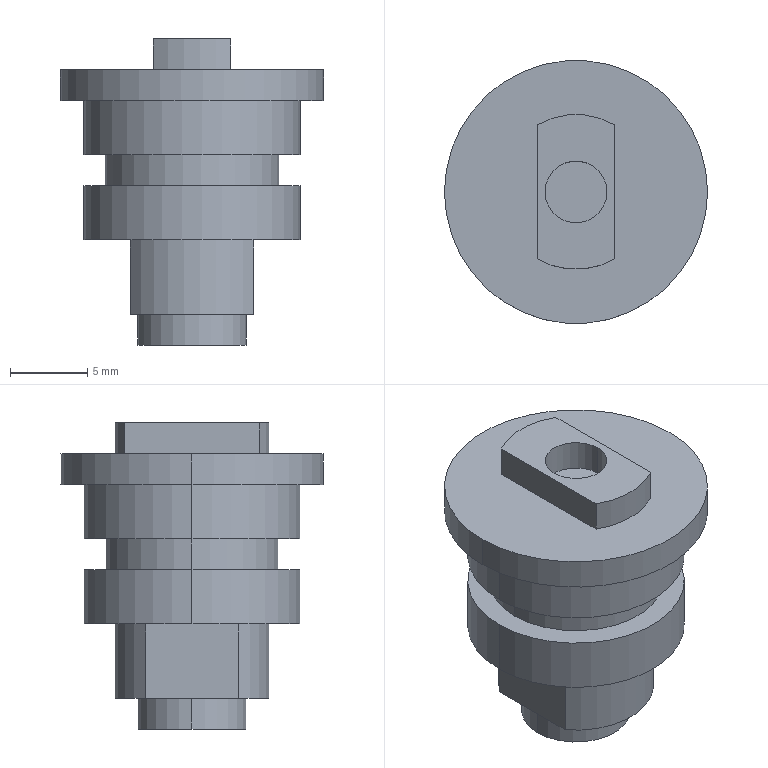Part | SolidWorks | features ICE 3, HoleWzd 1, Revolution 1 | 1 solid | 35 faces | box 17 x 17 x 19.8 mm | volume 2110 mm3 | cylinder 18 | plane 13 | cone 4 | commonest cylinder face diameters 10 x4 14 x4 4 x2 4.2 x2 7 x2 11.2 x2
STEP:
#1=CARTESIAN_POINT('',(-2.,0.,-2.));
#2=VERTEX_POINT('',#1);
#3=CARTESIAN_POINT('',(2.,0.,-2.));
#4=VERTEX_POINT('',#3);
#5=CARTESIAN_POINT('',(0.,0.,-2.));
#6=DIRECTION('',(0.,0.,1.));
#7=DIRECTION('',(1.,0.,0.));
#8=AXIS2_PLACEMENT_3D('',#5,#6,#7);
#9=CIRCLE('',#8,2.);
#10=EDGE_CURVE('',#2,#4,#9,.T.);
#11=ORIENTED_EDGE('',*,*,#10,.F.);
#12=CARTESIAN_POINT('',(-2.,0.,0.));
#13=VERTEX_POINT('',#12);
#14=CARTESIAN_POINT('',(-2.,0.,-2.));
#15=DIRECTION('',(0.,0.,1.));
#16=VECTOR('',#15,1000.);
#17=LINE('',#14,#16);
#18=EDGE_CURVE('',#2,#13,#17,.T.);
#19=ORIENTED_EDGE('',*,*,#18,.T.);
#20=CARTESIAN_POINT('',(2.,0.,0.));
#21=VERTEX_POINT('',#20);
#22=CARTESIAN_POINT('',(0.,0.,0.));
#23=DIRECTION('',(0.,0.,1.));
#24=DIRECTION('',(1.,0.,0.));
#25=AXIS2_PLACEMENT_3D('',#22,#23,#24);
#26=CIRCLE('',#25,2.);
#27=EDGE_CURVE('',#13,#21,#26,.T.);
#28=ORIENTED_EDGE('',*,*,#27,.T.);
#29=CARTESIAN_POINT('',(2.,0.,-2.));
#30=DIRECTION('',(0.,0.,1.));
#31=VECTOR('',#30,1000.);
#32=LINE('',#29,#31);
#33=EDGE_CURVE('',#4,#21,#32,.T.);
#34=ORIENTED_EDGE('',*,*,#33,.F.);
#35=EDGE_LOOP('',(#11,#19,#28,#34));
#36=FACE_OUTER_BOUND('',#35,.T.);
#37=CARTESIAN_POINT('',(0.,0.,-2.));
#38=DIRECTION('',(0.,0.,1.));
#39=DIRECTION('',(1.,0.,0.));
#40=AXIS2_PLACEMENT_3D('',#37,#38,#39);
#41=CYLINDRICAL_SURFACE('',#40,2.);
#42=ADVANCED_FACE('',(#36),#41,.F.);
#43=CARTESIAN_POINT('',(2.1,0.,-19.375));
#44=VERTEX_POINT('',#43);
#45=CARTESIAN_POINT('',(-2.1,0.,-19.375));
#46=VERTEX_POINT('',#45);
#47=CARTESIAN_POINT('',(0.,0.,-19.375));
#48=DIRECTION('',(0.,0.,-1.));
#49=DIRECTION('',(-1.,0.,0.));
#50=AXIS2_PLACEMENT_3D('',#47,#48,#49);
#51=CIRCLE('',#50,2.1);
#52=EDGE_CURVE('',#44,#46,#51,.T.);
#53=ORIENTED_EDGE('',*,*,#52,.F.);
#54=CARTESIAN_POINT('',(2.525,0.,-19.8));
#55=VERTEX_POINT('',#54);
#56=CARTESIAN_POINT('',(2.525,0.,-19.8));
#57=DIRECTION('',(0.7071,0.,-0.7071));
#58=VECTOR('',#57,1000.);
#59=LINE('',#56,#58);
#60=EDGE_CURVE('',#44,#55,#59,.T.);
#61=ORIENTED_EDGE('',*,*,#60,.T.);
#62=CARTESIAN_POINT('',(-2.525,0.,-19.8));
#63=VERTEX_POINT('',#62);
#64=CARTESIAN_POINT('',(0.,0.,-19.8));
#65=DIRECTION('',(0.,0.,-1.));
#66=DIRECTION('',(-1.,0.,0.));
#67=AXIS2_PLACEMENT_3D('',#64,#65,#66);
#68=CIRCLE('',#67,2.525);
#69=EDGE_CURVE('',#55,#63,#68,.T.);
#70=ORIENTED_EDGE('',*,*,#69,.T.);
#71=CARTESIAN_POINT('',(-2.525,0.,-19.8));
#72=DIRECTION('',(-0.7071,0.,-0.7071));
#73=VECTOR('',#72,1000.);
#74=LINE('',#71,#73);
#75=EDGE_CURVE('',#46,#63,#74,.T.);
#76=ORIENTED_EDGE('',*,*,#75,.F.);
#77=EDGE_LOOP('',(#53,#61,#70,#76));
#78=FACE_OUTER_BOUND('',#77,.T.);
#79=CARTESIAN_POINT('',(0.,0.,-19.8));
#80=DIRECTION('',(0.,0.,-1.));
#81=DIRECTION('',(-1.,0.,0.));
#82=AXIS2_PLACEMENT_3D('',#79,#80,#81);
#83=CONICAL_SURFACE('',#82,2.525,0.7854);
#84=ADVANCED_FACE('',(#78),#83,.F.);
#85=CARTESIAN_POINT('',(2.1,0.,-12.8));
#86=VERTEX_POINT('',#85);
#87=CARTESIAN_POINT('',(-2.1,0.,-12.8));
#88=VERTEX_POINT('',#87);
#89=CARTESIAN_POINT('',(0.,0.,-12.8));
#90=DIRECTION('',(0.,0.,-1.));
#91=DIRECTION('',(-1.,0.,0.));
#92=AXIS2_PLACEMENT_3D('',#89,#90,#91);
#93=CIRCLE('',#92,2.1);
#94=EDGE_CURVE('',#86,#88,#93,.T.);
#95=ORIENTED_EDGE('',*,*,#94,.F.);
#96=CARTESIAN_POINT('',(2.1,0.,-19.8));
#97=DIRECTION('',(0.,0.,-1.));
#98=VECTOR('',#97,1000.);
#99=LINE('',#96,#98);
#100=EDGE_CURVE('',#86,#44,#99,.T.);
#101=ORIENTED_EDGE('',*,*,#100,.T.);
#102=ORIENTED_EDGE('',*,*,#52,.T.);
#103=CARTESIAN_POINT('',(-2.1,0.,-19.8));
#104=DIRECTION('',(0.,0.,-1.));
#105=VECTOR('',#104,1000.);
#106=LINE('',#103,#105);
#107=EDGE_CURVE('',#88,#46,#106,.T.);
#108=ORIENTED_EDGE('',*,*,#107,.F.);
#109=EDGE_LOOP('',(#95,#101,#102,#108));
#110=FACE_OUTER_BOUND('',#109,.T.);
#111=CARTESIAN_POINT('',(0.,0.,-19.8));
#112=DIRECTION('',(0.,0.,-1.));
#113=DIRECTION('',(-1.,0.,0.));
#114=AXIS2_PLACEMENT_3D('',#111,#112,#113);
#115=CYLINDRICAL_SURFACE('',#114,2.1);
#116=ADVANCED_FACE('',(#110),#115,.F.);
#117=CARTESIAN_POINT('',(0.,0.,-11.538));
#118=VERTEX_POINT('',#117);
#119=CARTESIAN_POINT('',(-2.1,0.,-12.8));
#120=DIRECTION('',(-0.8572,0.,-0.515));
#121=VECTOR('',#120,1000.);
#122=LINE('',#119,#121);
#123=EDGE_CURVE('',#118,#88,#122,.T.);
#124=ORIENTED_EDGE('',*,*,#123,.F.);
#125=CARTESIAN_POINT('',(2.1,0.,-12.8));
#126=DIRECTION('',(0.8572,0.,-0.515));
#127=VECTOR('',#126,1000.);
#128=LINE('',#125,#127);
#129=EDGE_CURVE('',#118,#86,#128,.T.);
#130=ORIENTED_EDGE('',*,*,#129,.T.);
#131=ORIENTED_EDGE('',*,*,#94,.T.);
#132=EDGE_LOOP('',(#124,#130,#131));
#133=FACE_OUTER_BOUND('',#132,.T.);
#134=CARTESIAN_POINT('',(0.,0.,-12.8));
#135=DIRECTION('',(0.,0.,-1.));
#136=DIRECTION('',(-1.,0.,0.));
#137=AXIS2_PLACEMENT_3D('',#134,#135,#136);
#138=CONICAL_SURFACE('',#137,2.1,1.03);
#139=ADVANCED_FACE('',(#133),#138,.F.);
#140=CARTESIAN_POINT('',(-3.5,0.,-17.8));
#141=VERTEX_POINT('',#140);
#142=CARTESIAN_POINT('',(3.5,0.,-17.8));
#143=VERTEX_POINT('',#142);
#144=CARTESIAN_POINT('',(0.,0.,-17.8));
#145=DIRECTION('',(0.,0.,-1.));
#146=DIRECTION('',(-1.,0.,0.));
#147=AXIS2_PLACEMENT_3D('',#144,#145,#146);
#148=CIRCLE('',#147,3.5);
#149=EDGE_CURVE('',#141,#143,#148,.T.);
#150=ORIENTED_EDGE('',*,*,#149,.T.);
#151=CARTESIAN_POINT('',(3.5,0.,-19.8));
#152=VERTEX_POINT('',#151);
#153=CARTESIAN_POINT('',(3.5,0.,-19.8));
#154=DIRECTION('',(0.,0.,-1.));
#155=VECTOR('',#154,1000.);
#156=LINE('',#153,#155);
#157=EDGE_CURVE('',#143,#152,#156,.T.);
#158=ORIENTED_EDGE('',*,*,#157,.T.);
#159=CARTESIAN_POINT('',(-3.5,0.,-19.8));
#160=VERTEX_POINT('',#159);
#161=CARTESIAN_POINT('',(0.,0.,-19.8));
#162=DIRECTION('',(0.,0.,-1.));
#163=DIRECTION('',(-1.,0.,0.));
#164=AXIS2_PLACEMENT_3D('',#161,#162,#163);
#165=CIRCLE('',#164,3.5);
#166=EDGE_CURVE('',#160,#152,#165,.T.);
#167=ORIENTED_EDGE('',*,*,#166,.F.);
#168=CARTESIAN_POINT('',(-3.5,0.,-19.8));
#169=DIRECTION('',(0.,0.,-1.));
#170=VECTOR('',#169,1000.);
#171=LINE('',#168,#170);
#172=EDGE_CURVE('',#141,#160,#171,.T.);
#173=ORIENTED_EDGE('',*,*,#172,.F.);
#174=EDGE_LOOP('',(#150,#158,#167,#173));
#175=FACE_OUTER_BOUND('',#174,.T.);
#176=CARTESIAN_POINT('',(0.,0.,-19.8));
#177=DIRECTION('',(0.,0.,-1.));
#178=DIRECTION('',(-1.,0.,0.));
#179=AXIS2_PLACEMENT_3D('',#176,#177,#178);
#180=CYLINDRICAL_SURFACE('',#179,3.5);
#181=ADVANCED_FACE('',(#175),#180,.T.);
#182=CARTESIAN_POINT('',(-7.,0.,-9.5));
#183=VERTEX_POINT('',#182);
#184=CARTESIAN_POINT('',(7.,0.,-9.5));
#185=VERTEX_POINT('',#184);
#186=CARTESIAN_POINT('',(0.,0.,-9.5));
#187=DIRECTION('',(0.,0.,-1.));
#188=DIRECTION('',(-1.,0.,0.));
#189=AXIS2_PLACEMENT_3D('',#186,#187,#188);
#190=CIRCLE('',#189,7.);
#191=EDGE_CURVE('',#183,#185,#190,.T.);
#192=ORIENTED_EDGE('',*,*,#191,.T.);
#193=CARTESIAN_POINT('',(7.,0.,-13.));
#194=VERTEX_POINT('',#193);
#195=CARTESIAN_POINT('',(7.,0.,-19.8));
#196=DIRECTION('',(0.,0.,-1.));
#197=VECTOR('',#196,1000.);
#198=LINE('',#195,#197);
#199=EDGE_CURVE('',#185,#194,#198,.T.);
#200=ORIENTED_EDGE('',*,*,#199,.T.);
#201=CARTESIAN_POINT('',(-7.,0.,-13.));
#202=VERTEX_POINT('',#201);
#203=CARTESIAN_POINT('',(0.,0.,-13.));
#204=DIRECTION('',(0.,0.,-1.));
#205=DIRECTION('',(-1.,0.,0.));
#206=AXIS2_PLACEMENT_3D('',#203,#204,#205);
#207=CIRCLE('',#206,7.);
#208=EDGE_CURVE('',#202,#194,#207,.T.);
#209=ORIENTED_EDGE('',*,*,#208,.F.);
#210=CARTESIAN_POINT('',(-7.,0.,-19.8));
#211=DIRECTION('',(0.,0.,-1.));
#212=VECTOR('',#211,1000.);
#213=LINE('',#210,#212);
#214=EDGE_CURVE('',#183,#202,#213,.T.);
#215=ORIENTED_EDGE('',*,*,#214,.F.);
#216=EDGE_LOOP('',(#192,#200,#209,#215));
#217=FACE_OUTER_BOUND('',#216,.T.);
#218=CARTESIAN_POINT('',(0.,0.,-19.8));
#219=DIRECTION('',(0.,0.,-1.));
#220=DIRECTION('',(-1.,0.,0.));
#221=AXIS2_PLACEMENT_3D('',#218,#219,#220);
#222=CYLINDRICAL_SURFACE('',#221,7.);
#223=ADVANCED_FACE('',(#217),#222,.T.);
#224=CARTESIAN_POINT('',(-5.6,0.,-7.5));
#225=VERTEX_POINT('',#224);
#226=CARTESIAN_POINT('',(5.6,0.,-7.5));
#227=VERTEX_POINT('',#226);
#228=CARTESIAN_POINT('',(0.,0.,-7.5));
#229=DIRECTION('',(0.,0.,-1.));
#230=DIRECTION('',(-1.,0.,0.));
#231=AXIS2_PLACEMENT_3D('',#228,#229,#230);
#232=CIRCLE('',#231,5.6);
#233=EDGE_CURVE('',#225,#227,#232,.T.);
#234=ORIENTED_EDGE('',*,*,#233,.T.);
#235=CARTESIAN_POINT('',(5.6,0.,-9.5));
#236=VERTEX_POINT('',#235);
#237=CARTESIAN_POINT('',(5.6,0.,-19.8));
#238=DIRECTION('',(0.,0.,-1.));
#239=VECTOR('',#238,1000.);
#240=LINE('',#237,#239);
#241=EDGE_CURVE('',#227,#236,#240,.T.);
#242=ORIENTED_EDGE('',*,*,#241,.T.);
#243=CARTESIAN_POINT('',(-5.6,0.,-9.5));
#244=VERTEX_POINT('',#243);
#245=CARTESIAN_POINT('',(0.,0.,-9.5));
#246=DIRECTION('',(0.,0.,-1.));
#247=DIRECTION('',(-1.,0.,0.));
#248=AXIS2_PLACEMENT_3D('',#245,#246,#247);
#249=CIRCLE('',#248,5.6);
#250=EDGE_CURVE('',#244,#236,#249,.T.);
#251=ORIENTED_EDGE('',*,*,#250,.F.);
#252=CARTESIAN_POINT('',(-5.6,0.,-19.8));
#253=DIRECTION('',(0.,0.,-1.));
#254=VECTOR('',#253,1000.);
#255=LINE('',#252,#254);
#256=EDGE_CURVE('',#225,#244,#255,.T.);
#257=ORIENTED_EDGE('',*,*,#256,.F.);
#258=EDGE_LOOP('',(#234,#242,#251,#257));
#259=FACE_OUTER_BOUND('',#258,.T.);
#260=CARTESIAN_POINT('',(0.,0.,-19.8));
#261=DIRECTION('',(0.,0.,-1.));
#262=DIRECTION('',(-1.,0.,0.));
#263=AXIS2_PLACEMENT_3D('',#260,#261,#262);
#264=CYLINDRICAL_SURFACE('',#263,5.6);
#265=ADVANCED_FACE('',(#259),#264,.T.);
#266=CARTESIAN_POINT('',(-7.,0.,-4.));
#267=VERTEX_POINT('',#266);
#268=CARTESIAN_POINT('',(7.,0.,-4.));
#269=VERTEX_POINT('',#268);
#270=CARTESIAN_POINT('',(0.,0.,-4.));
#271=DIRECTION('',(0.,0.,-1.));
#272=DIRECTION('',(-1.,0.,0.));
#273=AXIS2_PLACEMENT_3D('',#270,#271,#272);
#274=CIRCLE('',#273,7.);
#275=EDGE_CURVE('',#267,#269,#274,.T.);
#276=ORIENTED_EDGE('',*,*,#275,.T.);
#277=CARTESIAN_POINT('',(7.,0.,-7.5));
#278=VERTEX_POINT('',#277);
#279=CARTESIAN_POINT('',(7.,0.,-19.8));
#280=DIRECTION('',(0.,0.,-1.));
#281=VECTOR('',#280,1000.);
#282=LINE('',#279,#281);
#283=EDGE_CURVE('',#269,#278,#282,.T.);
#284=ORIENTED_EDGE('',*,*,#283,.T.);
#285=CARTESIAN_POINT('',(-7.,0.,-7.5));
#286=VERTEX_POINT('',#285);
#287=CARTESIAN_POINT('',(0.,0.,-7.5));
#288=DIRECTION('',(0.,0.,-1.));
#289=DIRECTION('',(-1.,0.,0.));
#290=AXIS2_PLACEMENT_3D('',#287,#288,#289);
#291=CIRCLE('',#290,7.);
#292=EDGE_CURVE('',#286,#278,#291,.T.);
#293=ORIENTED_EDGE('',*,*,#292,.F.);
#294=CARTESIAN_POINT('',(-7.,0.,-19.8));
#295=DIRECTION('',(0.,0.,-1.));
#296=VECTOR('',#295,1000.);
#297=LINE('',#294,#296);
#298=EDGE_CURVE('',#267,#286,#297,.T.);
#299=ORIENTED_EDGE('',*,*,#298,.F.);
#300=EDGE_LOOP('',(#276,#284,#293,#299));
#301=FACE_OUTER_BOUND('',#300,.T.);
#302=CARTESIAN_POINT('',(0.,0.,-19.8));
#303=DIRECTION('',(0.,0.,-1.));
#304=DIRECTION('',(-1.,0.,0.));
#305=AXIS2_PLACEMENT_3D('',#302,#303,#304);
#306=CYLINDRICAL_SURFACE('',#305,7.);
#307=ADVANCED_FACE('',(#301),#306,.T.);
#308=CARTESIAN_POINT('',(-8.5,0.,-2.));
#309=VERTEX_POINT('',#308);
#310=CARTESIAN_POINT('',(8.5,0.,-2.));
#311=VERTEX_POINT('',#310);
#312=CARTESIAN_POINT('',(0.,0.,-2.));
#313=DIRECTION('',(0.,0.,-1.));
#314=DIRECTION('',(-1.,0.,0.));
#315=AXIS2_PLACEMENT_3D('',#312,#313,#314);
#316=CIRCLE('',#315,8.5);
#317=EDGE_CURVE('',#309,#311,#316,.T.);
#318=ORIENTED_EDGE('',*,*,#317,.T.);
#319=CARTESIAN_POINT('',(8.5,0.,-4.));
#320=VERTEX_POINT('',#319);
#321=CARTESIAN_POINT('',(8.5,0.,-19.8));
#322=DIRECTION('',(0.,0.,-1.));
#323=VECTOR('',#322,1000.);
#324=LINE('',#321,#323);
#325=EDGE_CURVE('',#311,#320,#324,.T.);
#326=ORIENTED_EDGE('',*,*,#325,.T.);
#327=CARTESIAN_POINT('',(-8.5,0.,-4.));
#328=VERTEX_POINT('',#327);
#329=CARTESIAN_POINT('',(0.,0.,-4.));
#330=DIRECTION('',(0.,0.,-1.));
#331=DIRECTION('',(-1.,0.,0.));
#332=AXIS2_PLACEMENT_3D('',#329,#330,#331);
#333=CIRCLE('',#332,8.5);
#334=EDGE_CURVE('',#328,#320,#333,.T.);
#335=ORIENTED_EDGE('',*,*,#334,.F.);
#336=CARTESIAN_POINT('',(-8.5,0.,-19.8));
#337=DIRECTION('',(0.,0.,-1.));
#338=VECTOR('',#337,1000.);
#339=LINE('',#336,#338);
#340=EDGE_CURVE('',#309,#328,#339,.T.);
#341=ORIENTED_EDGE('',*,*,#340,.F.);
#342=EDGE_LOOP('',(#318,#326,#335,#341));
#343=FACE_OUTER_BOUND('',#342,.T.);
#344=CARTESIAN_POINT('',(0.,0.,-19.8));
#345=DIRECTION('',(0.,0.,-1.));
#346=DIRECTION('',(-1.,0.,0.));
#347=AXIS2_PLACEMENT_3D('',#344,#345,#346);
#348=CYLINDRICAL_SURFACE('',#347,8.5);
#349=ADVANCED_FACE('',(#343),#348,.T.);
#350=CARTESIAN_POINT('',(4.,-3.,-17.8));
#351=VERTEX_POINT('',#350);
#352=CARTESIAN_POINT('',(-4.,-3.,-17.8));
#353=VERTEX_POINT('',#352);
#354=CARTESIAN_POINT('',(0.,0.,-17.8));
#355=DIRECTION('',(0.,0.,-1.));
#356=DIRECTION('',(-1.,0.,0.));
#357=AXIS2_PLACEMENT_3D('',#354,#355,#356);
#358=CIRCLE('',#357,5.);
#359=EDGE_CURVE('',#351,#353,#358,.T.);
#360=ORIENTED_EDGE('',*,*,#359,.F.);
#361=CARTESIAN_POINT('',(4.,-3.,-13.));
#362=VERTEX_POINT('',#361);
#363=CARTESIAN_POINT('',(4.,-3.,-19.8));
#364=DIRECTION('',(0.,0.,1.));
#365=VECTOR('',#364,1000.);
#366=LINE('',#363,#365);
#367=EDGE_CURVE('',#351,#362,#366,.T.);
#368=ORIENTED_EDGE('',*,*,#367,.T.);
#369=CARTESIAN_POINT('',(-4.,-3.,-13.));
#370=VERTEX_POINT('',#369);
#371=CARTESIAN_POINT('',(0.,0.,-13.));
#372=DIRECTION('',(0.,0.,-1.));
#373=DIRECTION('',(-1.,0.,0.));
#374=AXIS2_PLACEMENT_3D('',#371,#372,#373);
#375=CIRCLE('',#374,5.);
#376=EDGE_CURVE('',#362,#370,#375,.T.);
#377=ORIENTED_EDGE('',*,*,#376,.T.);
#378=CARTESIAN_POINT('',(-4.,-3.,-19.8));
#379=DIRECTION('',(0.,0.,-1.));
#380=VECTOR('',#379,1000.);
#381=LINE('',#378,#380);
#382=EDGE_CURVE('',#370,#353,#381,.T.);
#383=ORIENTED_EDGE('',*,*,#382,.T.);
#384=EDGE_LOOP('',(#360,#368,#377,#383));
#385=FACE_OUTER_BOUND('',#384,.T.);
#386=CARTESIAN_POINT('',(0.,0.,-19.8));
#387=DIRECTION('',(0.,0.,-1.));
#388=DIRECTION('',(-1.,0.,0.));
#389=AXIS2_PLACEMENT_3D('',#386,#387,#388);
#390=CYLINDRICAL_SURFACE('',#389,5.);
#391=ADVANCED_FACE('',(#385),#390,.T.);
#392=CARTESIAN_POINT('',(-4.,3.,-13.));
#393=VERTEX_POINT('',#392);
#394=CARTESIAN_POINT('',(4.,3.,-13.));
#395=VERTEX_POINT('',#394);
#396=CARTESIAN_POINT('',(0.,0.,-13.));
#397=DIRECTION('',(0.,0.,-1.));
#398=DIRECTION('',(-1.,0.,0.));
#399=AXIS2_PLACEMENT_3D('',#396,#397,#398);
#400=CIRCLE('',#399,5.);
#401=EDGE_CURVE('',#393,#395,#400,.T.);
#402=ORIENTED_EDGE('',*,*,#401,.T.);
#403=CARTESIAN_POINT('',(4.,3.,-17.8));
#404=VERTEX_POINT('',#403);
#405=CARTESIAN_POINT('',(4.,3.,-19.8));
#406=DIRECTION('',(0.,0.,-1.));
#407=VECTOR('',#406,1000.);
#408=LINE('',#405,#407);
#409=EDGE_CURVE('',#395,#404,#408,.T.);
#410=ORIENTED_EDGE('',*,*,#409,.T.);
#411=CARTESIAN_POINT('',(-4.,3.,-17.8));
#412=VERTEX_POINT('',#411);
#413=CARTESIAN_POINT('',(0.,0.,-17.8));
#414=DIRECTION('',(0.,0.,-1.));
#415=DIRECTION('',(-1.,0.,0.));
#416=AXIS2_PLACEMENT_3D('',#413,#414,#415);
#417=CIRCLE('',#416,5.);
#418=EDGE_CURVE('',#412,#404,#417,.T.);
#419=ORIENTED_EDGE('',*,*,#418,.F.);
#420=CARTESIAN_POINT('',(-4.,3.,-19.8));
#421=DIRECTION('',(0.,0.,1.));
#422=VECTOR('',#421,1000.);
#423=LINE('',#420,#422);
#424=EDGE_CURVE('',#412,#393,#423,.T.);
#425=ORIENTED_EDGE('',*,*,#424,.T.);
#426=EDGE_LOOP('',(#402,#410,#419,#425));
#427=FACE_OUTER_BOUND('',#426,.T.);
#428=CARTESIAN_POINT('',(0.,0.,-19.8));
#429=DIRECTION('',(0.,0.,-1.));
#430=DIRECTION('',(-1.,0.,0.));
#431=AXIS2_PLACEMENT_3D('',#428,#429,#430);
#432=CYLINDRICAL_SURFACE('',#431,5.);
#433=ADVANCED_FACE('',(#427),#432,.T.);
#434=ORIENTED_EDGE('',*,*,#149,.F.);
#435=CARTESIAN_POINT('',(0.,0.,-17.8));
#436=DIRECTION('',(0.,0.,-1.));
#437=DIRECTION('',(-1.,0.,0.));
#438=AXIS2_PLACEMENT_3D('',#435,#436,#437);
#439=CIRCLE('',#438,3.5);
#440=EDGE_CURVE('',#143,#141,#439,.T.);
#441=ORIENTED_EDGE('',*,*,#440,.F.);
#442=EDGE_LOOP('',(#434,#441));
#443=FACE_BOUND('',#442,.T.);
#444=ORIENTED_EDGE('',*,*,#418,.T.);
#445=CARTESIAN_POINT('',(4.,5.,-17.8));
#446=DIRECTION('',(0.,-1.,0.));
#447=VECTOR('',#446,1000.);
#448=LINE('',#445,#447);
#449=EDGE_CURVE('',#404,#351,#448,.T.);
#450=ORIENTED_EDGE('',*,*,#449,.T.);
#451=ORIENTED_EDGE('',*,*,#359,.T.);
#452=CARTESIAN_POINT('',(-4.,5.,-17.8));
#453=DIRECTION('',(0.,1.,0.));
#454=VECTOR('',#453,1000.);
#455=LINE('',#452,#454);
#456=EDGE_CURVE('',#353,#412,#455,.T.);
#457=ORIENTED_EDGE('',*,*,#456,.T.);
#458=EDGE_LOOP('',(#444,#450,#451,#457));
#459=FACE_OUTER_BOUND('',#458,.T.);
#460=CARTESIAN_POINT('',(0.,5.,-17.8));
#461=DIRECTION('',(0.,0.,-1.));
#462=DIRECTION('',(-1.,0.,0.));
#463=AXIS2_PLACEMENT_3D('',#460,#461,#462);
#464=PLANE('',#463);
#465=ADVANCED_FACE('',(#443,#459),#464,.T.);
#466=CARTESIAN_POINT('',(0.,0.,0.));
#467=DIRECTION('',(0.,0.,1.));
#468=DIRECTION('',(1.,0.,0.));
#469=AXIS2_PLACEMENT_3D('',#466,#467,#468);
#470=CIRCLE('',#469,2.);
#471=EDGE_CURVE('',#21,#13,#470,.T.);
#472=ORIENTED_EDGE('',*,*,#471,.F.);
#473=ORIENTED_EDGE('',*,*,#27,.F.);
#474=EDGE_LOOP('',(#472,#473));
#475=FACE_BOUND('',#474,.T.);
#476=CARTESIAN_POINT('',(-2.5,4.33,0.));
#477=VERTEX_POINT('',#476);
#478=CARTESIAN_POINT('',(2.5,4.33,0.));
#479=VERTEX_POINT('',#478);
#480=CARTESIAN_POINT('',(0.,0.,0.));
#481=DIRECTION('',(0.,0.,-1.));
#482=DIRECTION('',(-1.,0.,0.));
#483=AXIS2_PLACEMENT_3D('',#480,#481,#482);
#484=CIRCLE('',#483,5.);
#485=EDGE_CURVE('',#477,#479,#484,.T.);
#486=ORIENTED_EDGE('',*,*,#485,.F.);
#487=CARTESIAN_POINT('',(-2.5,-4.33,0.));
#488=VERTEX_POINT('',#487);
#489=CARTESIAN_POINT('',(-2.5,0.,0.));
#490=DIRECTION('',(0.,-1.,0.));
#491=VECTOR('',#490,1000.);
#492=LINE('',#489,#491);
#493=EDGE_CURVE('',#477,#488,#492,.T.);
#494=ORIENTED_EDGE('',*,*,#493,.T.);
#495=CARTESIAN_POINT('',(2.5,-4.33,0.));
#496=VERTEX_POINT('',#495);
#497=CARTESIAN_POINT('',(0.,0.,0.));
#498=DIRECTION('',(0.,0.,-1.));
#499=DIRECTION('',(-1.,0.,0.));
#500=AXIS2_PLACEMENT_3D('',#497,#498,#499);
#501=CIRCLE('',#500,5.);
#502=EDGE_CURVE('',#496,#488,#501,.T.);
#503=ORIENTED_EDGE('',*,*,#502,.F.);
#504=CARTESIAN_POINT('',(2.5,0.,0.));
#505=DIRECTION('',(0.,1.,0.));
#506=VECTOR('',#505,1000.);
#507=LINE('',#504,#506);
#508=EDGE_CURVE('',#496,#479,#507,.T.);
#509=ORIENTED_EDGE('',*,*,#508,.T.);
#510=EDGE_LOOP('',(#486,#494,#503,#509));
#511=FACE_OUTER_BOUND('',#510,.T.);
#512=CARTESIAN_POINT('',(0.,0.,0.));
#513=DIRECTION('',(0.,0.,1.));
#514=DIRECTION('',(1.,0.,0.));
#515=AXIS2_PLACEMENT_3D('',#512,#513,#514);
#516=PLANE('',#515);
#517=ADVANCED_FACE('',(#475,#511),#516,.T.);
#518=CARTESIAN_POINT('',(-2.5,4.33,-2.));
#519=VERTEX_POINT('',#518);
#520=CARTESIAN_POINT('',(2.5,4.33,-2.));
#521=VERTEX_POINT('',#520);
#522=CARTESIAN_POINT('',(0.,0.,-2.));
#523=DIRECTION('',(0.,0.,-1.));
#524=DIRECTION('',(-1.,0.,0.));
#525=AXIS2_PLACEMENT_3D('',#522,#523,#524);
#526=CIRCLE('',#525,5.);
#527=EDGE_CURVE('',#519,#521,#526,.T.);
#528=ORIENTED_EDGE('',*,*,#527,.F.);
#529=CARTESIAN_POINT('',(-2.5,4.33,-19.8));
#530=DIRECTION('',(0.,0.,1.));
#531=VECTOR('',#530,1000.);
#532=LINE('',#529,#531);
#533=EDGE_CURVE('',#519,#477,#532,.T.);
#534=ORIENTED_EDGE('',*,*,#533,.T.);
#535=ORIENTED_EDGE('',*,*,#485,.T.);
#536=CARTESIAN_POINT('',(2.5,4.33,-19.8));
#537=DIRECTION('',(0.,0.,-1.));
#538=VECTOR('',#537,1000.);
#539=LINE('',#536,#538);
#540=EDGE_CURVE('',#479,#521,#539,.T.);
#541=ORIENTED_EDGE('',*,*,#540,.T.);
#542=EDGE_LOOP('',(#528,#534,#535,#541));
#543=FACE_OUTER_BOUND('',#542,.T.);
#544=CARTESIAN_POINT('',(0.,0.,-19.8));
#545=DIRECTION('',(0.,0.,-1.));
#546=DIRECTION('',(-1.,0.,0.));
#547=AXIS2_PLACEMENT_3D('',#544,#545,#546);
#548=CYLINDRICAL_SURFACE('',#547,5.);
#549=ADVANCED_FACE('',(#543),#548,.T.);
#550=ORIENTED_EDGE('',*,*,#502,.T.);
#551=CARTESIAN_POINT('',(-2.5,-4.33,-2.));
#552=VERTEX_POINT('',#551);
#553=CARTESIAN_POINT('',(-2.5,-4.33,-19.8));
#554=DIRECTION('',(0.,0.,-1.));
#555=VECTOR('',#554,1000.);
#556=LINE('',#553,#555);
#557=EDGE_CURVE('',#488,#552,#556,.T.);
#558=ORIENTED_EDGE('',*,*,#557,.T.);
#559=CARTESIAN_POINT('',(2.5,-4.33,-2.));
#560=VERTEX_POINT('',#559);
#561=CARTESIAN_POINT('',(0.,0.,-2.));
#562=DIRECTION('',(0.,0.,-1.));
#563=DIRECTION('',(-1.,0.,0.));
#564=AXIS2_PLACEMENT_3D('',#561,#562,#563);
#565=CIRCLE('',#564,5.);
#566=EDGE_CURVE('',#560,#552,#565,.T.);
#567=ORIENTED_EDGE('',*,*,#566,.F.);
#568=CARTESIAN_POINT('',(2.5,-4.33,-19.8));
#569=DIRECTION('',(0.,0.,1.));
#570=VECTOR('',#569,1000.);
#571=LINE('',#568,#570);
#572=EDGE_CURVE('',#560,#496,#571,.T.);
#573=ORIENTED_EDGE('',*,*,#572,.T.);
#574=EDGE_LOOP('',(#550,#558,#567,#573));
#575=FACE_OUTER_BOUND('',#574,.T.);
#576=CARTESIAN_POINT('',(0.,0.,-19.8));
#577=DIRECTION('',(0.,0.,-1.));
#578=DIRECTION('',(-1.,0.,0.));
#579=AXIS2_PLACEMENT_3D('',#576,#577,#578);
#580=CYLINDRICAL_SURFACE('',#579,5.);
#581=ADVANCED_FACE('',(#575),#580,.T.);
#582=ORIENTED_EDGE('',*,*,#566,.T.);
#583=CARTESIAN_POINT('',(-2.5,-17.202,-2.));
#584=DIRECTION('',(0.,1.,0.));
#585=VECTOR('',#584,1000.);
#586=LINE('',#583,#585);
#587=EDGE_CURVE('',#552,#519,#586,.T.);
#588=ORIENTED_EDGE('',*,*,#587,.T.);
#589=ORIENTED_EDGE('',*,*,#527,.T.);
#590=CARTESIAN_POINT('',(2.5,-17.202,-2.));
#591=DIRECTION('',(0.,-1.,0.));
#592=VECTOR('',#591,1000.);
#593=LINE('',#590,#592);
#594=EDGE_CURVE('',#521,#560,#593,.T.);
#595=ORIENTED_EDGE('',*,*,#594,.T.);
#596=EDGE_LOOP('',(#582,#588,#589,#595));
#597=FACE_BOUND('',#596,.T.);
#598=ORIENTED_EDGE('',*,*,#317,.F.);
#599=CARTESIAN_POINT('',(0.,0.,-2.));
#600=DIRECTION('',(0.,0.,-1.));
#601=DIRECTION('',(-1.,0.,0.));
#602=AXIS2_PLACEMENT_3D('',#599,#600,#601);
#603=CIRCLE('',#602,8.5);
#604=EDGE_CURVE('',#311,#309,#603,.T.);
#605=ORIENTED_EDGE('',*,*,#604,.F.);
#606=EDGE_LOOP('',(#598,#605));
#607=FACE_OUTER_BOUND('',#606,.T.);
#608=CARTESIAN_POINT('',(0.,5.,-2.));
#609=DIRECTION('',(0.,0.,1.));
#610=DIRECTION('',(1.,0.,0.));
#611=AXIS2_PLACEMENT_3D('',#608,#609,#610);
#612=PLANE('',#611);
#613=ADVANCED_FACE('',(#597,#607),#612,.T.);
#614=ORIENTED_EDGE('',*,*,#325,.F.);
#615=ORIENTED_EDGE('',*,*,#604,.T.);
#616=ORIENTED_EDGE('',*,*,#340,.T.);
#617=CARTESIAN_POINT('',(0.,0.,-4.));
#618=DIRECTION('',(0.,0.,-1.));
#619=DIRECTION('',(-1.,0.,0.));
#620=AXIS2_PLACEMENT_3D('',#617,#618,#619);
#621=CIRCLE('',#620,8.5);
#622=EDGE_CURVE('',#320,#328,#621,.T.);
#623=ORIENTED_EDGE('',*,*,#622,.F.);
#624=EDGE_LOOP('',(#614,#615,#616,#623));
#625=FACE_OUTER_BOUND('',#624,.T.);
#626=CARTESIAN_POINT('',(0.,0.,-19.8));
#627=DIRECTION('',(0.,0.,-1.));
#628=DIRECTION('',(-1.,0.,0.));
#629=AXIS2_PLACEMENT_3D('',#626,#627,#628);
#630=CYLINDRICAL_SURFACE('',#629,8.5);
#631=ADVANCED_FACE('',(#625),#630,.T.);
#632=ORIENTED_EDGE('',*,*,#334,.T.);
#633=ORIENTED_EDGE('',*,*,#622,.T.);
#634=EDGE_LOOP('',(#632,#633));
#635=FACE_OUTER_BOUND('',#634,.T.);
#636=ORIENTED_EDGE('',*,*,#275,.F.);
#637=CARTESIAN_POINT('',(0.,0.,-4.));
#638=DIRECTION('',(0.,0.,-1.));
#639=DIRECTION('',(-1.,0.,0.));
#640=AXIS2_PLACEMENT_3D('',#637,#638,#639);
#641=CIRCLE('',#640,7.);
#642=EDGE_CURVE('',#269,#267,#641,.T.);
#643=ORIENTED_EDGE('',*,*,#642,.F.);
#644=EDGE_LOOP('',(#636,#643));
#645=FACE_BOUND('',#644,.T.);
#646=CARTESIAN_POINT('',(0.,8.5,-4.));
#647=DIRECTION('',(0.,0.,-1.));
#648=DIRECTION('',(-1.,0.,0.));
#649=AXIS2_PLACEMENT_3D('',#646,#647,#648);
#650=PLANE('',#649);
#651=ADVANCED_FACE('',(#635,#645),#650,.T.);
#652=ORIENTED_EDGE('',*,*,#283,.F.);
#653=ORIENTED_EDGE('',*,*,#642,.T.);
#654=ORIENTED_EDGE('',*,*,#298,.T.);
#655=CARTESIAN_POINT('',(0.,0.,-7.5));
#656=DIRECTION('',(0.,0.,-1.));
#657=DIRECTION('',(-1.,0.,0.));
#658=AXIS2_PLACEMENT_3D('',#655,#656,#657);
#659=CIRCLE('',#658,7.);
#660=EDGE_CURVE('',#278,#286,#659,.T.);
#661=ORIENTED_EDGE('',*,*,#660,.F.);
#662=EDGE_LOOP('',(#652,#653,#654,#661));
#663=FACE_OUTER_BOUND('',#662,.T.);
#664=CARTESIAN_POINT('',(0.,0.,-19.8));
#665=DIRECTION('',(0.,0.,-1.));
#666=DIRECTION('',(-1.,0.,0.));
#667=AXIS2_PLACEMENT_3D('',#664,#665,#666);
#668=CYLINDRICAL_SURFACE('',#667,7.);
#669=ADVANCED_FACE('',(#663),#668,.T.);
#670=ORIENTED_EDGE('',*,*,#292,.T.);
#671=ORIENTED_EDGE('',*,*,#660,.T.);
#672=EDGE_LOOP('',(#670,#671));
#673=FACE_OUTER_BOUND('',#672,.T.);
#674=ORIENTED_EDGE('',*,*,#233,.F.);
#675=CARTESIAN_POINT('',(0.,0.,-7.5));
#676=DIRECTION('',(0.,0.,-1.));
#677=DIRECTION('',(-1.,0.,0.));
#678=AXIS2_PLACEMENT_3D('',#675,#676,#677);
#679=CIRCLE('',#678,5.6);
#680=EDGE_CURVE('',#227,#225,#679,.T.);
#681=ORIENTED_EDGE('',*,*,#680,.F.);
#682=EDGE_LOOP('',(#674,#681));
#683=FACE_BOUND('',#682,.T.);
#684=CARTESIAN_POINT('',(0.,7.,-7.5));
#685=DIRECTION('',(0.,0.,-1.));
#686=DIRECTION('',(-1.,0.,0.));
#687=AXIS2_PLACEMENT_3D('',#684,#685,#686);
#688=PLANE('',#687);
#689=ADVANCED_FACE('',(#673,#683),#688,.T.);
#690=ORIENTED_EDGE('',*,*,#241,.F.);
#691=ORIENTED_EDGE('',*,*,#680,.T.);
#692=ORIENTED_EDGE('',*,*,#256,.T.);
#693=CARTESIAN_POINT('',(0.,0.,-9.5));
#694=DIRECTION('',(0.,0.,-1.));
#695=DIRECTION('',(-1.,0.,0.));
#696=AXIS2_PLACEMENT_3D('',#693,#694,#695);
#697=CIRCLE('',#696,5.6);
#698=EDGE_CURVE('',#236,#244,#697,.T.);
#699=ORIENTED_EDGE('',*,*,#698,.F.);
#700=EDGE_LOOP('',(#690,#691,#692,#699));
#701=FACE_OUTER_BOUND('',#700,.T.);
#702=CARTESIAN_POINT('',(0.,0.,-19.8));
#703=DIRECTION('',(0.,0.,-1.));
#704=DIRECTION('',(-1.,0.,0.));
#705=AXIS2_PLACEMENT_3D('',#702,#703,#704);
#706=CYLINDRICAL_SURFACE('',#705,5.6);
#707=ADVANCED_FACE('',(#701),#706,.T.);
#708=ORIENTED_EDGE('',*,*,#250,.T.);
#709=ORIENTED_EDGE('',*,*,#698,.T.);
#710=EDGE_LOOP('',(#708,#709));
#711=FACE_BOUND('',#710,.T.);
#712=ORIENTED_EDGE('',*,*,#191,.F.);
#713=CARTESIAN_POINT('',(0.,0.,-9.5));
#714=DIRECTION('',(0.,0.,-1.));
#715=DIRECTION('',(-1.,0.,0.));
#716=AXIS2_PLACEMENT_3D('',#713,#714,#715);
#717=CIRCLE('',#716,7.);
#718=EDGE_CURVE('',#185,#183,#717,.T.);
#719=ORIENTED_EDGE('',*,*,#718,.F.);
#720=EDGE_LOOP('',(#712,#719));
#721=FACE_OUTER_BOUND('',#720,.T.);
#722=CARTESIAN_POINT('',(0.,5.6,-9.5));
#723=DIRECTION('',(0.,0.,1.));
#724=DIRECTION('',(1.,0.,0.));
#725=AXIS2_PLACEMENT_3D('',#722,#723,#724);
#726=PLANE('',#725);
#727=ADVANCED_FACE('',(#711,#721),#726,.T.);
#728=ORIENTED_EDGE('',*,*,#199,.F.);
#729=ORIENTED_EDGE('',*,*,#718,.T.);
#730=ORIENTED_EDGE('',*,*,#214,.T.);
#731=CARTESIAN_POINT('',(0.,0.,-13.));
#732=DIRECTION('',(0.,0.,-1.));
#733=DIRECTION('',(-1.,0.,0.));
#734=AXIS2_PLACEMENT_3D('',#731,#732,#733);
#735=CIRCLE('',#734,7.);
#736=EDGE_CURVE('',#194,#202,#735,.T.);
#737=ORIENTED_EDGE('',*,*,#736,.F.);
#738=EDGE_LOOP('',(#728,#729,#730,#737));
#739=FACE_OUTER_BOUND('',#738,.T.);
#740=CARTESIAN_POINT('',(0.,0.,-19.8));
#741=DIRECTION('',(0.,0.,-1.));
#742=DIRECTION('',(-1.,0.,0.));
#743=AXIS2_PLACEMENT_3D('',#740,#741,#742);
#744=CYLINDRICAL_SURFACE('',#743,7.);
#745=ADVANCED_FACE('',(#739),#744,.T.);
#746=CARTESIAN_POINT('',(4.,-11.657,-13.));
#747=DIRECTION('',(0.,1.,0.));
#748=VECTOR('',#747,1000.);
#749=LINE('',#746,#748);
#750=EDGE_CURVE('',#362,#395,#749,.T.);
#751=ORIENTED_EDGE('',*,*,#750,.T.);
#752=ORIENTED_EDGE('',*,*,#401,.F.);
#753=CARTESIAN_POINT('',(-4.,-11.657,-13.));
#754=DIRECTION('',(0.,-1.,0.));
#755=VECTOR('',#754,1000.);
#756=LINE('',#753,#755);
#757=EDGE_CURVE('',#393,#370,#756,.T.);
#758=ORIENTED_EDGE('',*,*,#757,.T.);
#759=ORIENTED_EDGE('',*,*,#376,.F.);
#760=EDGE_LOOP('',(#751,#752,#758,#759));
#761=FACE_BOUND('',#760,.T.);
#762=ORIENTED_EDGE('',*,*,#208,.T.);
#763=ORIENTED_EDGE('',*,*,#736,.T.);
#764=EDGE_LOOP('',(#762,#763));
#765=FACE_OUTER_BOUND('',#764,.T.);
#766=CARTESIAN_POINT('',(0.,7.,-13.));
#767=DIRECTION('',(0.,0.,-1.));
#768=DIRECTION('',(-1.,0.,0.));
#769=AXIS2_PLACEMENT_3D('',#766,#767,#768);
#770=PLANE('',#769);
#771=ADVANCED_FACE('',(#761,#765),#770,.T.);
#772=ORIENTED_EDGE('',*,*,#157,.F.);
#773=ORIENTED_EDGE('',*,*,#440,.T.);
#774=ORIENTED_EDGE('',*,*,#172,.T.);
#775=CARTESIAN_POINT('',(0.,0.,-19.8));
#776=DIRECTION('',(0.,0.,-1.));
#777=DIRECTION('',(-1.,0.,0.));
#778=AXIS2_PLACEMENT_3D('',#775,#776,#777);
#779=CIRCLE('',#778,3.5);
#780=EDGE_CURVE('',#152,#160,#779,.T.);
#781=ORIENTED_EDGE('',*,*,#780,.F.);
#782=EDGE_LOOP('',(#772,#773,#774,#781));
#783=FACE_OUTER_BOUND('',#782,.T.);
#784=CARTESIAN_POINT('',(0.,0.,-19.8));
#785=DIRECTION('',(0.,0.,-1.));
#786=DIRECTION('',(-1.,0.,0.));
#787=AXIS2_PLACEMENT_3D('',#784,#785,#786);
#788=CYLINDRICAL_SURFACE('',#787,3.5);
#789=ADVANCED_FACE('',(#783),#788,.T.);
#790=CARTESIAN_POINT('',(0.,0.,-19.8));
#791=DIRECTION('',(0.,0.,-1.));
#792=DIRECTION('',(-1.,0.,0.));
#793=AXIS2_PLACEMENT_3D('',#790,#791,#792);
#794=CIRCLE('',#793,2.525);
#795=EDGE_CURVE('',#63,#55,#794,.T.);
#796=ORIENTED_EDGE('',*,*,#795,.F.);
#797=ORIENTED_EDGE('',*,*,#69,.F.);
#798=EDGE_LOOP('',(#796,#797));
#799=FACE_BOUND('',#798,.T.);
#800=ORIENTED_EDGE('',*,*,#166,.T.);
#801=ORIENTED_EDGE('',*,*,#780,.T.);
#802=EDGE_LOOP('',(#800,#801));
#803=FACE_OUTER_BOUND('',#802,.T.);
#804=CARTESIAN_POINT('',(0.,3.5,-19.8));
#805=DIRECTION('',(0.,0.,-1.));
#806=DIRECTION('',(-1.,0.,0.));
#807=AXIS2_PLACEMENT_3D('',#804,#805,#806);
#808=PLANE('',#807);
#809=ADVANCED_FACE('',(#799,#803),#808,.T.);
#810=ORIENTED_EDGE('',*,*,#594,.F.);
#811=ORIENTED_EDGE('',*,*,#540,.F.);
#812=ORIENTED_EDGE('',*,*,#508,.F.);
#813=ORIENTED_EDGE('',*,*,#572,.F.);
#814=EDGE_LOOP('',(#810,#811,#812,#813));
#815=FACE_OUTER_BOUND('',#814,.T.);
#816=CARTESIAN_POINT('',(2.5,-17.202,-41.695));
#817=DIRECTION('',(1.,0.,0.));
#818=DIRECTION('',(0.,0.,-1.));
#819=AXIS2_PLACEMENT_3D('',#816,#817,#818);
#820=PLANE('',#819);
#821=ADVANCED_FACE('',(#815),#820,.T.);
#822=ORIENTED_EDGE('',*,*,#587,.F.);
#823=ORIENTED_EDGE('',*,*,#557,.F.);
#824=ORIENTED_EDGE('',*,*,#493,.F.);
#825=ORIENTED_EDGE('',*,*,#533,.F.);
#826=EDGE_LOOP('',(#822,#823,#824,#825));
#827=FACE_OUTER_BOUND('',#826,.T.);
#828=CARTESIAN_POINT('',(-2.5,-17.202,-41.695));
#829=DIRECTION('',(-1.,0.,0.));
#830=DIRECTION('',(0.,0.,1.));
#831=AXIS2_PLACEMENT_3D('',#828,#829,#830);
#832=PLANE('',#831);
#833=ADVANCED_FACE('',(#827),#832,.T.);
#834=ORIENTED_EDGE('',*,*,#456,.F.);
#835=ORIENTED_EDGE('',*,*,#382,.F.);
#836=ORIENTED_EDGE('',*,*,#757,.F.);
#837=ORIENTED_EDGE('',*,*,#424,.F.);
#838=EDGE_LOOP('',(#834,#835,#836,#837));
#839=FACE_OUTER_BOUND('',#838,.T.);
#840=CARTESIAN_POINT('',(-4.,-11.657,17.019));
#841=DIRECTION('',(-1.,0.,0.));
#842=DIRECTION('',(0.,0.,1.));
#843=AXIS2_PLACEMENT_3D('',#840,#841,#842);
#844=PLANE('',#843);
#845=ADVANCED_FACE('',(#839),#844,.T.);
#846=ORIENTED_EDGE('',*,*,#449,.F.);
#847=ORIENTED_EDGE('',*,*,#409,.F.);
#848=ORIENTED_EDGE('',*,*,#750,.F.);
#849=ORIENTED_EDGE('',*,*,#367,.F.);
#850=EDGE_LOOP('',(#846,#847,#848,#849));
#851=FACE_OUTER_BOUND('',#850,.T.);
#852=CARTESIAN_POINT('',(4.,-11.657,17.019));
#853=DIRECTION('',(1.,0.,0.));
#854=DIRECTION('',(0.,0.,-1.));
#855=AXIS2_PLACEMENT_3D('',#852,#853,#854);
#856=PLANE('',#855);
#857=ADVANCED_FACE('',(#851),#856,.T.);
#858=ORIENTED_EDGE('',*,*,#129,.F.);
#859=ORIENTED_EDGE('',*,*,#123,.T.);
#860=CARTESIAN_POINT('',(0.,0.,-12.8));
#861=DIRECTION('',(0.,0.,-1.));
#862=DIRECTION('',(-1.,0.,0.));
#863=AXIS2_PLACEMENT_3D('',#860,#861,#862);
#864=CIRCLE('',#863,2.1);
#865=EDGE_CURVE('',#88,#86,#864,.T.);
#866=ORIENTED_EDGE('',*,*,#865,.T.);
#867=EDGE_LOOP('',(#858,#859,#866));
#868=FACE_OUTER_BOUND('',#867,.T.);
#869=CARTESIAN_POINT('',(0.,0.,-12.8));
#870=DIRECTION('',(0.,0.,-1.));
#871=DIRECTION('',(-1.,0.,0.));
#872=AXIS2_PLACEMENT_3D('',#869,#870,#871);
#873=CONICAL_SURFACE('',#872,2.1,1.03);
#874=ADVANCED_FACE('',(#868),#873,.F.);
#875=ORIENTED_EDGE('',*,*,#100,.F.);
#876=ORIENTED_EDGE('',*,*,#865,.F.);
#877=ORIENTED_EDGE('',*,*,#107,.T.);
#878=CARTESIAN_POINT('',(0.,0.,-19.375));
#879=DIRECTION('',(0.,0.,-1.));
#880=DIRECTION('',(-1.,0.,0.));
#881=AXIS2_PLACEMENT_3D('',#878,#879,#880);
#882=CIRCLE('',#881,2.1);
#883=EDGE_CURVE('',#46,#44,#882,.T.);
#884=ORIENTED_EDGE('',*,*,#883,.T.);
#885=EDGE_LOOP('',(#875,#876,#877,#884));
#886=FACE_OUTER_BOUND('',#885,.T.);
#887=CARTESIAN_POINT('',(0.,0.,-19.8));
#888=DIRECTION('',(0.,0.,-1.));
#889=DIRECTION('',(-1.,0.,0.));
#890=AXIS2_PLACEMENT_3D('',#887,#888,#889);
#891=CYLINDRICAL_SURFACE('',#890,2.1);
#892=ADVANCED_FACE('',(#886),#891,.F.);
#893=ORIENTED_EDGE('',*,*,#60,.F.);
#894=ORIENTED_EDGE('',*,*,#883,.F.);
#895=ORIENTED_EDGE('',*,*,#75,.T.);
#896=ORIENTED_EDGE('',*,*,#795,.T.);
#897=EDGE_LOOP('',(#893,#894,#895,#896));
#898=FACE_OUTER_BOUND('',#897,.T.);
#899=CARTESIAN_POINT('',(0.,0.,-19.8));
#900=DIRECTION('',(0.,0.,-1.));
#901=DIRECTION('',(-1.,0.,0.));
#902=AXIS2_PLACEMENT_3D('',#899,#900,#901);
#903=CONICAL_SURFACE('',#902,2.525,0.7854);
#904=ADVANCED_FACE('',(#898),#903,.F.);
#905=ORIENTED_EDGE('',*,*,#18,.F.);
#906=CARTESIAN_POINT('',(0.,0.,-2.));
#907=DIRECTION('',(0.,0.,1.));
#908=DIRECTION('',(1.,0.,0.));
#909=AXIS2_PLACEMENT_3D('',#906,#907,#908);
#910=CIRCLE('',#909,2.);
#911=EDGE_CURVE('',#4,#2,#910,.T.);
#912=ORIENTED_EDGE('',*,*,#911,.F.);
#913=ORIENTED_EDGE('',*,*,#33,.T.);
#914=ORIENTED_EDGE('',*,*,#471,.T.);
#915=EDGE_LOOP('',(#905,#912,#913,#914));
#916=FACE_OUTER_BOUND('',#915,.T.);
#917=CARTESIAN_POINT('',(0.,0.,-2.));
#918=DIRECTION('',(0.,0.,1.));
#919=DIRECTION('',(1.,0.,0.));
#920=AXIS2_PLACEMENT_3D('',#917,#918,#919);
#921=CYLINDRICAL_SURFACE('',#920,2.);
#922=ADVANCED_FACE('',(#916),#921,.F.);
#923=ORIENTED_EDGE('',*,*,#911,.T.);
#924=ORIENTED_EDGE('',*,*,#10,.T.);
#925=EDGE_LOOP('',(#923,#924));
#926=FACE_OUTER_BOUND('',#925,.T.);
#927=CARTESIAN_POINT('',(0.,0.,-2.));
#928=DIRECTION('',(0.,0.,1.));
#929=DIRECTION('',(1.,0.,0.));
#930=AXIS2_PLACEMENT_3D('',#927,#928,#929);
#931=PLANE('',#930);
#932=ADVANCED_FACE('',(#926),#931,.T.);
#933=CLOSED_SHELL('',(#42,#84,#116,#139,#181,#223,#265,#307,#349,#391,#433,#465,#517,#549,#581,#613,#631,#651,#669,#689,#707,#727,#745,#771,#789,#809,#821,#833,#845,#857,#874,#892,#904,#922,#932));
#934=MANIFOLD_SOLID_BREP('',#933);
#935=CARTESIAN_POINT('',(0.,0.,0.));
#936=DIRECTION('',(0.,0.,1.));
#937=DIRECTION('',(1.,0.,0.));
#938=AXIS2_PLACEMENT_3D('',#935,#936,#937);
#939=(LENGTH_UNIT()NAMED_UNIT(*)SI_UNIT(.MILLI.,.METRE.));
#940=UNCERTAINTY_MEASURE_WITH_UNIT(LENGTH_MEASURE(0.00001),#939,'','');
#941=(NAMED_UNIT(*)PLANE_ANGLE_UNIT()SI_UNIT($,.RADIAN.));
#942=(NAMED_UNIT(*)SI_UNIT($,.STERADIAN.)SOLID_ANGLE_UNIT());
#943=(GEOMETRIC_REPRESENTATION_CONTEXT(3)GLOBAL_UNCERTAINTY_ASSIGNED_CONTEXT((#940))GLOBAL_UNIT_ASSIGNED_CONTEXT((#939,#941,#942))REPRESENTATION_CONTEXT('',''));
#944=ADVANCED_BREP_SHAPE_REPRESENTATION('',(#934,#938),#943);